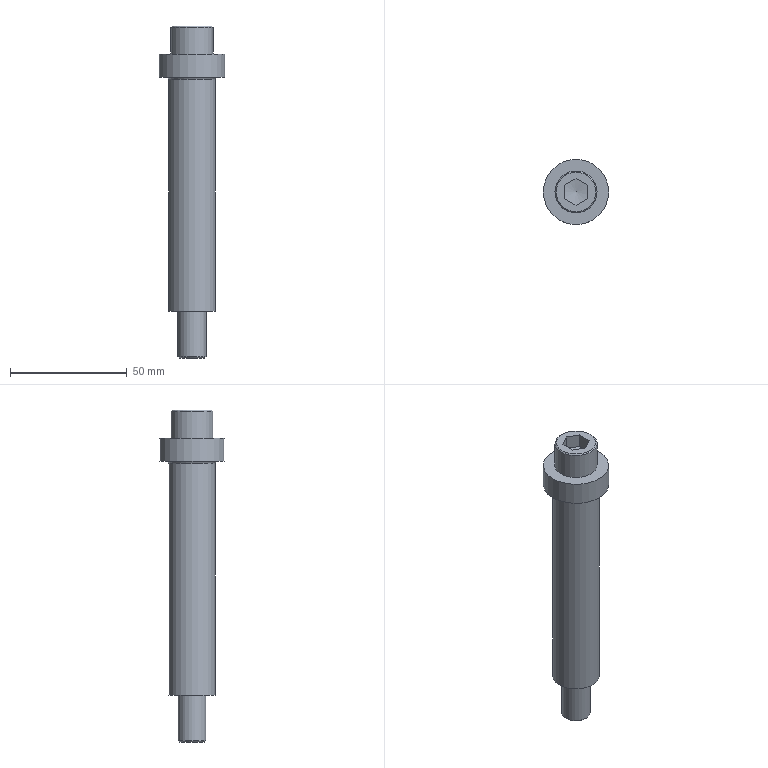Part | NX | features CSR20-100_1 2 | 1 solid | 27 faces | box 28 x 28 x 142 mm | volume 41062 mm3 | plane 18 | cylinder 5 | cone 3 | torus 1 | commonest cylinder face diameters 12 x1 12.6 x1 18 x1 20 x1 28 x1
STEP:
#1=CARTESIAN_POINT('',(1485.899,-26.667,139.999));
#2=VERTEX_POINT('',#1);
#3=CARTESIAN_POINT('',(1471.899,-26.667,139.999));
#4=DIRECTION('',(0.,0.,-1.));
#5=DIRECTION('',(1.,0.,0.));
#6=AXIS2_PLACEMENT_3D('',#3,#4,#5);
#7=CIRCLE('',#6,14.);
#8=EDGE_CURVE('',#2,#2,#7,.T.);
#9=ORIENTED_EDGE('',*,*,#8,.F.);
#10=EDGE_LOOP('',(#9));
#11=FACE_BOUND('',#10,.T.);
#12=CARTESIAN_POINT('',(1480.899,-26.667,139.999));
#13=VERTEX_POINT('',#12);
#14=CARTESIAN_POINT('',(1471.899,-26.667,139.999));
#15=DIRECTION('',(0.,0.,1.));
#16=DIRECTION('',(1.,0.,0.));
#17=AXIS2_PLACEMENT_3D('',#14,#15,#16);
#18=CIRCLE('',#17,9.);
#19=EDGE_CURVE('',#13,#13,#18,.T.);
#20=ORIENTED_EDGE('',*,*,#19,.F.);
#21=EDGE_LOOP('',(#20));
#22=FACE_BOUND('',#21,.T.);
#23=CARTESIAN_POINT('',(1471.899,-26.667,139.999));
#24=DIRECTION('',(0.,0.,1.));
#25=DIRECTION('',(1.,0.,0.));
#26=AXIS2_PLACEMENT_3D('',#23,#24,#25);
#27=PLANE('',#26);
#28=ADVANCED_FACE('',(#11,#22),#27,.T.);
#29=CARTESIAN_POINT('',(1481.899,-26.667,29.999));
#30=VERTEX_POINT('',#29);
#31=CARTESIAN_POINT('',(1471.899,-26.667,29.999));
#32=DIRECTION('',(0.,0.,1.));
#33=DIRECTION('',(1.,0.,0.));
#34=AXIS2_PLACEMENT_3D('',#31,#32,#33);
#35=CIRCLE('',#34,10.);
#36=EDGE_CURVE('',#30,#30,#35,.T.);
#37=ORIENTED_EDGE('',*,*,#36,.T.);
#38=EDGE_LOOP('',(#37));
#39=FACE_BOUND('',#38,.T.);
#40=CARTESIAN_POINT('',(1481.899,-26.667,128.999));
#41=VERTEX_POINT('',#40);
#42=CARTESIAN_POINT('',(1471.899,-26.667,128.999));
#43=DIRECTION('',(0.,0.,-1.));
#44=DIRECTION('',(-1.,0.,0.));
#45=AXIS2_PLACEMENT_3D('',#42,#43,#44);
#46=CIRCLE('',#45,10.);
#47=EDGE_CURVE('',#41,#41,#46,.T.);
#48=ORIENTED_EDGE('',*,*,#47,.T.);
#49=EDGE_LOOP('',(#48));
#50=FACE_BOUND('',#49,.T.);
#51=CARTESIAN_POINT('',(1471.899,-26.667,79.999));
#52=DIRECTION('',(0.,0.,-1.));
#53=DIRECTION('',(-1.,0.,0.));
#54=AXIS2_PLACEMENT_3D('',#51,#52,#53);
#55=CYLINDRICAL_SURFACE('',#54,10.);
#56=ADVANCED_FACE('',(#39,#50),#55,.T.);
#57=CARTESIAN_POINT('',(1478.199,-26.667,139.999));
#58=VERTEX_POINT('',#57);
#59=CARTESIAN_POINT('',(1471.899,-26.667,139.999));
#60=DIRECTION('',(0.,0.,1.));
#61=DIRECTION('',(1.,0.,0.));
#62=AXIS2_PLACEMENT_3D('',#59,#60,#61);
#63=CIRCLE('',#62,6.3);
#64=EDGE_CURVE('',#58,#58,#63,.T.);
#65=ORIENTED_EDGE('',*,*,#64,.T.);
#66=EDGE_LOOP('',(#65));
#67=FACE_BOUND('',#66,.T.);
#68=CARTESIAN_POINT('',(1478.199,-26.667,29.999));
#69=VERTEX_POINT('',#68);
#70=CARTESIAN_POINT('',(1471.899,-26.667,29.999));
#71=DIRECTION('',(0.,0.,-1.));
#72=DIRECTION('',(1.,0.,0.));
#73=AXIS2_PLACEMENT_3D('',#70,#71,#72);
#74=CIRCLE('',#73,6.3);
#75=EDGE_CURVE('',#69,#69,#74,.T.);
#76=ORIENTED_EDGE('',*,*,#75,.T.);
#77=EDGE_LOOP('',(#76));
#78=FACE_BOUND('',#77,.T.);
#79=CARTESIAN_POINT('',(1471.899,-26.667,84.999));
#80=DIRECTION('',(0.,0.,-1.));
#81=DIRECTION('',(-1.,0.,0.));
#82=AXIS2_PLACEMENT_3D('',#79,#80,#81);
#83=CYLINDRICAL_SURFACE('',#82,6.3);
#84=ADVANCED_FACE('',(#67,#78),#83,.F.);
#85=ORIENTED_EDGE('',*,*,#47,.F.);
#86=EDGE_LOOP('',(#85));
#87=FACE_BOUND('',#86,.T.);
#88=CARTESIAN_POINT('',(1482.899,-26.667,129.999));
#89=VERTEX_POINT('',#88);
#90=CARTESIAN_POINT('',(1471.899,-26.667,129.999));
#91=DIRECTION('',(0.,0.,1.));
#92=DIRECTION('',(-1.,0.,0.));
#93=AXIS2_PLACEMENT_3D('',#90,#91,#92);
#94=CIRCLE('',#93,11.);
#95=EDGE_CURVE('',#89,#89,#94,.T.);
#96=ORIENTED_EDGE('',*,*,#95,.F.);
#97=EDGE_LOOP('',(#96));
#98=FACE_BOUND('',#97,.T.);
#99=CARTESIAN_POINT('',(1471.899,-26.667,128.999));
#100=DIRECTION('',(0.,0.,1.));
#101=DIRECTION('',(1.,0.,0.));
#102=AXIS2_PLACEMENT_3D('',#99,#100,#101);
#103=TOROIDAL_SURFACE('',#102,11.,1.);
#104=ADVANCED_FACE('',(#87,#98),#103,.F.);
#105=CARTESIAN_POINT('',(1485.899,-26.667,129.999));
#106=VERTEX_POINT('',#105);
#107=CARTESIAN_POINT('',(1471.899,-26.667,129.999));
#108=DIRECTION('',(0.,0.,1.));
#109=DIRECTION('',(1.,0.,0.));
#110=AXIS2_PLACEMENT_3D('',#107,#108,#109);
#111=CIRCLE('',#110,14.);
#112=EDGE_CURVE('',#106,#106,#111,.T.);
#113=ORIENTED_EDGE('',*,*,#112,.F.);
#114=EDGE_LOOP('',(#113));
#115=FACE_BOUND('',#114,.T.);
#116=ORIENTED_EDGE('',*,*,#95,.T.);
#117=EDGE_LOOP('',(#116));
#118=FACE_BOUND('',#117,.T.);
#119=CARTESIAN_POINT('',(1471.899,-26.667,129.999));
#120=DIRECTION('',(0.,0.,-1.));
#121=DIRECTION('',(-1.,0.,0.));
#122=AXIS2_PLACEMENT_3D('',#119,#120,#121);
#123=PLANE('',#122);
#124=ADVANCED_FACE('',(#115,#118),#123,.T.);
#125=ORIENTED_EDGE('',*,*,#75,.F.);
#126=EDGE_LOOP('',(#125));
#127=FACE_BOUND('',#126,.T.);
#128=ORIENTED_EDGE('',*,*,#36,.F.);
#129=EDGE_LOOP('',(#128));
#130=FACE_BOUND('',#129,.T.);
#131=CARTESIAN_POINT('',(1471.899,-26.667,29.999));
#132=DIRECTION('',(0.,0.,-1.));
#133=DIRECTION('',(-1.,0.,0.));
#134=AXIS2_PLACEMENT_3D('',#131,#132,#133);
#135=PLANE('',#134);
#136=ADVANCED_FACE('',(#127,#130),#135,.T.);
#137=ORIENTED_EDGE('',*,*,#8,.T.);
#138=EDGE_LOOP('',(#137));
#139=FACE_BOUND('',#138,.T.);
#140=ORIENTED_EDGE('',*,*,#112,.T.);
#141=EDGE_LOOP('',(#140));
#142=FACE_BOUND('',#141,.T.);
#143=CARTESIAN_POINT('',(1471.899,-26.667,134.999));
#144=DIRECTION('',(0.,0.,-1.));
#145=DIRECTION('',(-1.,0.,0.));
#146=AXIS2_PLACEMENT_3D('',#143,#144,#145);
#147=CYLINDRICAL_SURFACE('',#146,14.);
#148=ADVANCED_FACE('',(#139,#142),#147,.T.);
#149=CARTESIAN_POINT('',(1471.899,-32.441,151.999));
#150=VERTEX_POINT('',#149);
#151=CARTESIAN_POINT('',(1476.899,-29.554,151.999));
#152=VERTEX_POINT('',#151);
#153=CARTESIAN_POINT('',(1474.399,-30.997,151.999));
#154=DIRECTION('',(0.866,0.5,0.));
#155=VECTOR('',#154,1000.);
#156=LINE('',#153,#155);
#157=EDGE_CURVE('',#150,#152,#156,.T.);
#158=ORIENTED_EDGE('',*,*,#157,.F.);
#159=CARTESIAN_POINT('',(1466.899,-29.554,151.999));
#160=VERTEX_POINT('',#159);
#161=CARTESIAN_POINT('',(1469.399,-30.997,151.999));
#162=DIRECTION('',(0.866,-0.5,0.));
#163=VECTOR('',#162,1000.);
#164=LINE('',#161,#163);
#165=EDGE_CURVE('',#160,#150,#164,.T.);
#166=ORIENTED_EDGE('',*,*,#165,.F.);
#167=CARTESIAN_POINT('',(1466.899,-23.78,151.999));
#168=VERTEX_POINT('',#167);
#169=CARTESIAN_POINT('',(1466.899,-26.667,151.999));
#170=DIRECTION('',(0.,-1.,0.));
#171=VECTOR('',#170,1000.);
#172=LINE('',#169,#171);
#173=EDGE_CURVE('',#168,#160,#172,.T.);
#174=ORIENTED_EDGE('',*,*,#173,.F.);
#175=CARTESIAN_POINT('',(1471.899,-20.894,151.999));
#176=VERTEX_POINT('',#175);
#177=CARTESIAN_POINT('',(1469.399,-22.337,151.999));
#178=DIRECTION('',(-0.866,-0.5,0.));
#179=VECTOR('',#178,1000.);
#180=LINE('',#177,#179);
#181=EDGE_CURVE('',#176,#168,#180,.T.);
#182=ORIENTED_EDGE('',*,*,#181,.F.);
#183=CARTESIAN_POINT('',(1476.899,-23.78,151.999));
#184=VERTEX_POINT('',#183);
#185=CARTESIAN_POINT('',(1474.399,-22.337,151.999));
#186=DIRECTION('',(-0.866,0.5,0.));
#187=VECTOR('',#186,1000.);
#188=LINE('',#185,#187);
#189=EDGE_CURVE('',#184,#176,#188,.T.);
#190=ORIENTED_EDGE('',*,*,#189,.F.);
#191=CARTESIAN_POINT('',(1476.899,-26.667,151.999));
#192=DIRECTION('',(0.,1.,0.));
#193=VECTOR('',#192,1000.);
#194=LINE('',#191,#193);
#195=EDGE_CURVE('',#152,#184,#194,.T.);
#196=ORIENTED_EDGE('',*,*,#195,.F.);
#197=EDGE_LOOP('',(#158,#166,#174,#182,#190,#196));
#198=FACE_BOUND('',#197,.T.);
#199=CARTESIAN_POINT('',(1480.399,-26.667,151.999));
#200=VERTEX_POINT('',#199);
#201=CARTESIAN_POINT('',(1471.899,-26.667,151.999));
#202=DIRECTION('',(0.,0.,1.));
#203=DIRECTION('',(-1.,0.,0.));
#204=AXIS2_PLACEMENT_3D('',#201,#202,#203);
#205=CIRCLE('',#204,8.5);
#206=EDGE_CURVE('',#200,#200,#205,.T.);
#207=ORIENTED_EDGE('',*,*,#206,.T.);
#208=EDGE_LOOP('',(#207));
#209=FACE_BOUND('',#208,.T.);
#210=CARTESIAN_POINT('',(1471.899,-26.667,151.999));
#211=DIRECTION('',(0.,0.,1.));
#212=DIRECTION('',(1.,0.,0.));
#213=AXIS2_PLACEMENT_3D('',#210,#211,#212);
#214=PLANE('',#213);
#215=ADVANCED_FACE('',(#198,#209),#214,.T.);
#216=ORIENTED_EDGE('',*,*,#19,.T.);
#217=EDGE_LOOP('',(#216));
#218=FACE_BOUND('',#217,.T.);
#219=CARTESIAN_POINT('',(1480.899,-26.667,151.499));
#220=VERTEX_POINT('',#219);
#221=CARTESIAN_POINT('',(1471.899,-26.667,151.499));
#222=DIRECTION('',(0.,0.,-1.));
#223=DIRECTION('',(-1.,0.,0.));
#224=AXIS2_PLACEMENT_3D('',#221,#222,#223);
#225=CIRCLE('',#224,9.);
#226=EDGE_CURVE('',#220,#220,#225,.T.);
#227=ORIENTED_EDGE('',*,*,#226,.T.);
#228=EDGE_LOOP('',(#227));
#229=FACE_BOUND('',#228,.T.);
#230=CARTESIAN_POINT('',(1471.899,-26.667,145.999));
#231=DIRECTION('',(0.,0.,-1.));
#232=DIRECTION('',(-1.,0.,0.));
#233=AXIS2_PLACEMENT_3D('',#230,#231,#232);
#234=CYLINDRICAL_SURFACE('',#233,9.);
#235=ADVANCED_FACE('',(#218,#229),#234,.T.);
#236=ORIENTED_EDGE('',*,*,#226,.F.);
#237=EDGE_LOOP('',(#236));
#238=FACE_BOUND('',#237,.T.);
#239=ORIENTED_EDGE('',*,*,#206,.F.);
#240=EDGE_LOOP('',(#239));
#241=FACE_BOUND('',#240,.T.);
#242=CARTESIAN_POINT('',(1471.899,-26.667,151.999));
#243=DIRECTION('',(0.,0.,-1.));
#244=DIRECTION('',(1.,0.,0.));
#245=AXIS2_PLACEMENT_3D('',#242,#243,#244);
#246=CONICAL_SURFACE('',#245,8.5,0.7854);
#247=ADVANCED_FACE('',(#238,#241),#246,.T.);
#248=CARTESIAN_POINT('',(1476.899,-29.554,145.999));
#249=VERTEX_POINT('',#248);
#250=CARTESIAN_POINT('',(1476.899,-29.554,148.999));
#251=DIRECTION('',(0.,0.,1.));
#252=VECTOR('',#251,1000.);
#253=LINE('',#250,#252);
#254=EDGE_CURVE('',#249,#152,#253,.T.);
#255=ORIENTED_EDGE('',*,*,#254,.T.);
#256=ORIENTED_EDGE('',*,*,#195,.T.);
#257=CARTESIAN_POINT('',(1476.899,-23.78,145.999));
#258=VERTEX_POINT('',#257);
#259=CARTESIAN_POINT('',(1476.899,-23.78,148.999));
#260=DIRECTION('',(0.,0.,1.));
#261=VECTOR('',#260,1000.);
#262=LINE('',#259,#261);
#263=EDGE_CURVE('',#258,#184,#262,.T.);
#264=ORIENTED_EDGE('',*,*,#263,.F.);
#265=CARTESIAN_POINT('',(1476.899,-26.667,145.999));
#266=DIRECTION('',(0.,1.,0.));
#267=VECTOR('',#266,1000.);
#268=LINE('',#265,#267);
#269=EDGE_CURVE('',#249,#258,#268,.T.);
#270=ORIENTED_EDGE('',*,*,#269,.F.);
#271=EDGE_LOOP('',(#255,#256,#264,#270));
#272=FACE_BOUND('',#271,.T.);
#273=CARTESIAN_POINT('',(1476.899,-26.667,148.999));
#274=DIRECTION('',(-1.,0.,0.));
#275=DIRECTION('',(0.,0.,1.));
#276=AXIS2_PLACEMENT_3D('',#273,#274,#275);
#277=PLANE('',#276);
#278=ADVANCED_FACE('',(#272),#277,.T.);
#279=ORIENTED_EDGE('',*,*,#263,.T.);
#280=ORIENTED_EDGE('',*,*,#189,.T.);
#281=CARTESIAN_POINT('',(1471.899,-20.894,145.999));
#282=VERTEX_POINT('',#281);
#283=CARTESIAN_POINT('',(1471.899,-20.894,148.999));
#284=DIRECTION('',(0.,0.,1.));
#285=VECTOR('',#284,1000.);
#286=LINE('',#283,#285);
#287=EDGE_CURVE('',#282,#176,#286,.T.);
#288=ORIENTED_EDGE('',*,*,#287,.F.);
#289=CARTESIAN_POINT('',(1474.399,-22.337,145.999));
#290=DIRECTION('',(-0.866,0.5,0.));
#291=VECTOR('',#290,1000.);
#292=LINE('',#289,#291);
#293=EDGE_CURVE('',#258,#282,#292,.T.);
#294=ORIENTED_EDGE('',*,*,#293,.F.);
#295=EDGE_LOOP('',(#279,#280,#288,#294));
#296=FACE_BOUND('',#295,.T.);
#297=CARTESIAN_POINT('',(1474.399,-22.337,148.999));
#298=DIRECTION('',(-0.5,-0.866,0.));
#299=DIRECTION('',(0.,0.,1.));
#300=AXIS2_PLACEMENT_3D('',#297,#298,#299);
#301=PLANE('',#300);
#302=ADVANCED_FACE('',(#296),#301,.T.);
#303=ORIENTED_EDGE('',*,*,#287,.T.);
#304=ORIENTED_EDGE('',*,*,#181,.T.);
#305=CARTESIAN_POINT('',(1466.899,-23.78,145.999));
#306=VERTEX_POINT('',#305);
#307=CARTESIAN_POINT('',(1466.899,-23.78,148.999));
#308=DIRECTION('',(0.,0.,1.));
#309=VECTOR('',#308,1000.);
#310=LINE('',#307,#309);
#311=EDGE_CURVE('',#306,#168,#310,.T.);
#312=ORIENTED_EDGE('',*,*,#311,.F.);
#313=CARTESIAN_POINT('',(1469.399,-22.337,145.999));
#314=DIRECTION('',(-0.866,-0.5,0.));
#315=VECTOR('',#314,1000.);
#316=LINE('',#313,#315);
#317=EDGE_CURVE('',#282,#306,#316,.T.);
#318=ORIENTED_EDGE('',*,*,#317,.F.);
#319=EDGE_LOOP('',(#303,#304,#312,#318));
#320=FACE_BOUND('',#319,.T.);
#321=CARTESIAN_POINT('',(1469.399,-22.337,148.999));
#322=DIRECTION('',(0.5,-0.866,0.));
#323=DIRECTION('',(0.,0.,-1.));
#324=AXIS2_PLACEMENT_3D('',#321,#322,#323);
#325=PLANE('',#324);
#326=ADVANCED_FACE('',(#320),#325,.T.);
#327=ORIENTED_EDGE('',*,*,#311,.T.);
#328=ORIENTED_EDGE('',*,*,#173,.T.);
#329=CARTESIAN_POINT('',(1466.899,-29.554,145.999));
#330=VERTEX_POINT('',#329);
#331=CARTESIAN_POINT('',(1466.899,-29.554,148.999));
#332=DIRECTION('',(0.,0.,1.));
#333=VECTOR('',#332,1000.);
#334=LINE('',#331,#333);
#335=EDGE_CURVE('',#330,#160,#334,.T.);
#336=ORIENTED_EDGE('',*,*,#335,.F.);
#337=CARTESIAN_POINT('',(1466.899,-26.667,145.999));
#338=DIRECTION('',(0.,-1.,0.));
#339=VECTOR('',#338,1000.);
#340=LINE('',#337,#339);
#341=EDGE_CURVE('',#306,#330,#340,.T.);
#342=ORIENTED_EDGE('',*,*,#341,.F.);
#343=EDGE_LOOP('',(#327,#328,#336,#342));
#344=FACE_BOUND('',#343,.T.);
#345=CARTESIAN_POINT('',(1466.899,-26.667,148.999));
#346=DIRECTION('',(1.,0.,0.));
#347=DIRECTION('',(0.,0.,-1.));
#348=AXIS2_PLACEMENT_3D('',#345,#346,#347);
#349=PLANE('',#348);
#350=ADVANCED_FACE('',(#344),#349,.T.);
#351=ORIENTED_EDGE('',*,*,#335,.T.);
#352=ORIENTED_EDGE('',*,*,#165,.T.);
#353=CARTESIAN_POINT('',(1471.899,-32.441,145.999));
#354=VERTEX_POINT('',#353);
#355=CARTESIAN_POINT('',(1471.899,-32.441,148.999));
#356=DIRECTION('',(0.,0.,1.));
#357=VECTOR('',#356,1000.);
#358=LINE('',#355,#357);
#359=EDGE_CURVE('',#354,#150,#358,.T.);
#360=ORIENTED_EDGE('',*,*,#359,.F.);
#361=CARTESIAN_POINT('',(1469.399,-30.997,145.999));
#362=DIRECTION('',(0.866,-0.5,0.));
#363=VECTOR('',#362,1000.);
#364=LINE('',#361,#363);
#365=EDGE_CURVE('',#330,#354,#364,.T.);
#366=ORIENTED_EDGE('',*,*,#365,.F.);
#367=EDGE_LOOP('',(#351,#352,#360,#366));
#368=FACE_BOUND('',#367,.T.);
#369=CARTESIAN_POINT('',(1469.399,-30.997,148.999));
#370=DIRECTION('',(0.5,0.866,0.));
#371=DIRECTION('',(0.,0.,-1.));
#372=AXIS2_PLACEMENT_3D('',#369,#370,#371);
#373=PLANE('',#372);
#374=ADVANCED_FACE('',(#368),#373,.T.);
#375=ORIENTED_EDGE('',*,*,#359,.T.);
#376=ORIENTED_EDGE('',*,*,#157,.T.);
#377=ORIENTED_EDGE('',*,*,#254,.F.);
#378=CARTESIAN_POINT('',(1474.399,-30.997,145.999));
#379=DIRECTION('',(0.866,0.5,0.));
#380=VECTOR('',#379,1000.);
#381=LINE('',#378,#380);
#382=EDGE_CURVE('',#354,#249,#381,.T.);
#383=ORIENTED_EDGE('',*,*,#382,.F.);
#384=EDGE_LOOP('',(#375,#376,#377,#383));
#385=FACE_BOUND('',#384,.T.);
#386=CARTESIAN_POINT('',(1474.399,-30.997,148.999));
#387=DIRECTION('',(-0.5,0.866,0.));
#388=DIRECTION('',(0.,0.,1.));
#389=AXIS2_PLACEMENT_3D('',#386,#387,#388);
#390=PLANE('',#389);
#391=ADVANCED_FACE('',(#385),#390,.T.);
#392=CARTESIAN_POINT('',(1471.899,-26.667,145.999));
#393=DIRECTION('',(0.,0.,-1.));
#394=DIRECTION('',(1.,0.,0.));
#395=AXIS2_PLACEMENT_3D('',#392,#393,#394);
#396=CIRCLE('',#395,5.774);
#397=EDGE_CURVE('',#258,#249,#396,.T.);
#398=ORIENTED_EDGE('',*,*,#397,.F.);
#399=CARTESIAN_POINT('',(1471.899,-26.667,145.999));
#400=DIRECTION('',(0.,0.,-1.));
#401=DIRECTION('',(1.,0.,0.));
#402=AXIS2_PLACEMENT_3D('',#399,#400,#401);
#403=CIRCLE('',#402,5.774);
#404=EDGE_CURVE('',#282,#258,#403,.T.);
#405=ORIENTED_EDGE('',*,*,#404,.F.);
#406=CARTESIAN_POINT('',(1471.899,-26.667,145.999));
#407=DIRECTION('',(0.,0.,-1.));
#408=DIRECTION('',(1.,0.,0.));
#409=AXIS2_PLACEMENT_3D('',#406,#407,#408);
#410=CIRCLE('',#409,5.774);
#411=EDGE_CURVE('',#306,#282,#410,.T.);
#412=ORIENTED_EDGE('',*,*,#411,.F.);
#413=CARTESIAN_POINT('',(1471.899,-26.667,145.999));
#414=DIRECTION('',(0.,0.,-1.));
#415=DIRECTION('',(1.,0.,0.));
#416=AXIS2_PLACEMENT_3D('',#413,#414,#415);
#417=CIRCLE('',#416,5.774);
#418=EDGE_CURVE('',#330,#306,#417,.T.);
#419=ORIENTED_EDGE('',*,*,#418,.F.);
#420=CARTESIAN_POINT('',(1471.899,-26.667,145.999));
#421=DIRECTION('',(0.,0.,-1.));
#422=DIRECTION('',(1.,0.,0.));
#423=AXIS2_PLACEMENT_3D('',#420,#421,#422);
#424=CIRCLE('',#423,5.774);
#425=EDGE_CURVE('',#354,#330,#424,.T.);
#426=ORIENTED_EDGE('',*,*,#425,.F.);
#427=CARTESIAN_POINT('',(1471.899,-26.667,145.999));
#428=DIRECTION('',(0.,0.,-1.));
#429=DIRECTION('',(1.,0.,0.));
#430=AXIS2_PLACEMENT_3D('',#427,#428,#429);
#431=CIRCLE('',#430,5.774);
#432=EDGE_CURVE('',#249,#354,#431,.T.);
#433=ORIENTED_EDGE('',*,*,#432,.F.);
#434=EDGE_LOOP('',(#398,#405,#412,#419,#426,#433));
#435=FACE_BOUND('',#434,.T.);
#436=CARTESIAN_POINT('',(1471.899,-26.667,144.999));
#437=VERTEX_POINT('',#436);
#438=VERTEX_LOOP('',#437);
#439=FACE_BOUND('',#438,.T.);
#440=CARTESIAN_POINT('',(1471.899,-26.667,145.499));
#441=DIRECTION('',(0.,0.,1.));
#442=DIRECTION('',(-1.,0.,0.));
#443=AXIS2_PLACEMENT_3D('',#440,#441,#442);
#444=CONICAL_SURFACE('',#443,2.887,1.399);
#445=ADVANCED_FACE('',(#435,#439),#444,.F.);
#446=ORIENTED_EDGE('',*,*,#365,.T.);
#447=ORIENTED_EDGE('',*,*,#425,.T.);
#448=EDGE_LOOP('',(#446,#447));
#449=FACE_BOUND('',#448,.T.);
#450=CARTESIAN_POINT('',(1471.899,-26.667,145.999));
#451=DIRECTION('',(0.,0.,1.));
#452=DIRECTION('',(1.,0.,0.));
#453=AXIS2_PLACEMENT_3D('',#450,#451,#452);
#454=PLANE('',#453);
#455=ADVANCED_FACE('',(#449),#454,.F.);
#456=ORIENTED_EDGE('',*,*,#341,.T.);
#457=ORIENTED_EDGE('',*,*,#418,.T.);
#458=EDGE_LOOP('',(#456,#457));
#459=FACE_BOUND('',#458,.T.);
#460=CARTESIAN_POINT('',(1471.899,-26.667,145.999));
#461=DIRECTION('',(0.,0.,1.));
#462=DIRECTION('',(1.,0.,0.));
#463=AXIS2_PLACEMENT_3D('',#460,#461,#462);
#464=PLANE('',#463);
#465=ADVANCED_FACE('',(#459),#464,.F.);
#466=ORIENTED_EDGE('',*,*,#317,.T.);
#467=ORIENTED_EDGE('',*,*,#411,.T.);
#468=EDGE_LOOP('',(#466,#467));
#469=FACE_BOUND('',#468,.T.);
#470=CARTESIAN_POINT('',(1471.899,-26.667,145.999));
#471=DIRECTION('',(0.,0.,1.));
#472=DIRECTION('',(1.,0.,0.));
#473=AXIS2_PLACEMENT_3D('',#470,#471,#472);
#474=PLANE('',#473);
#475=ADVANCED_FACE('',(#469),#474,.F.);
#476=ORIENTED_EDGE('',*,*,#293,.T.);
#477=ORIENTED_EDGE('',*,*,#404,.T.);
#478=EDGE_LOOP('',(#476,#477));
#479=FACE_BOUND('',#478,.T.);
#480=CARTESIAN_POINT('',(1471.899,-26.667,145.999));
#481=DIRECTION('',(0.,0.,1.));
#482=DIRECTION('',(1.,0.,0.));
#483=AXIS2_PLACEMENT_3D('',#480,#481,#482);
#484=PLANE('',#483);
#485=ADVANCED_FACE('',(#479),#484,.F.);
#486=ORIENTED_EDGE('',*,*,#269,.T.);
#487=ORIENTED_EDGE('',*,*,#397,.T.);
#488=EDGE_LOOP('',(#486,#487));
#489=FACE_BOUND('',#488,.T.);
#490=CARTESIAN_POINT('',(1471.899,-26.667,145.999));
#491=DIRECTION('',(0.,0.,1.));
#492=DIRECTION('',(1.,0.,0.));
#493=AXIS2_PLACEMENT_3D('',#490,#491,#492);
#494=PLANE('',#493);
#495=ADVANCED_FACE('',(#489),#494,.F.);
#496=ORIENTED_EDGE('',*,*,#382,.T.);
#497=ORIENTED_EDGE('',*,*,#432,.T.);
#498=EDGE_LOOP('',(#496,#497));
#499=FACE_BOUND('',#498,.T.);
#500=CARTESIAN_POINT('',(1471.899,-26.667,145.999));
#501=DIRECTION('',(0.,0.,1.));
#502=DIRECTION('',(1.,0.,0.));
#503=AXIS2_PLACEMENT_3D('',#500,#501,#502);
#504=PLANE('',#503);
#505=ADVANCED_FACE('',(#499),#504,.F.);
#506=CARTESIAN_POINT('',(1477.899,-26.667,10.499));
#507=VERTEX_POINT('',#506);
#508=CARTESIAN_POINT('',(1471.899,-26.667,10.499));
#509=DIRECTION('',(0.,0.,1.));
#510=DIRECTION('',(-1.,0.,0.));
#511=AXIS2_PLACEMENT_3D('',#508,#509,#510);
#512=CIRCLE('',#511,6.);
#513=EDGE_CURVE('',#507,#507,#512,.T.);
#514=ORIENTED_EDGE('',*,*,#513,.F.);
#515=EDGE_LOOP('',(#514));
#516=FACE_BOUND('',#515,.T.);
#517=CARTESIAN_POINT('',(1477.399,-26.667,9.999));
#518=VERTEX_POINT('',#517);
#519=CARTESIAN_POINT('',(1471.899,-26.667,9.999));
#520=DIRECTION('',(0.,0.,-1.));
#521=DIRECTION('',(-1.,0.,0.));
#522=AXIS2_PLACEMENT_3D('',#519,#520,#521);
#523=CIRCLE('',#522,5.5);
#524=EDGE_CURVE('',#518,#518,#523,.T.);
#525=ORIENTED_EDGE('',*,*,#524,.F.);
#526=EDGE_LOOP('',(#525));
#527=FACE_BOUND('',#526,.T.);
#528=CARTESIAN_POINT('',(1471.899,-26.667,9.999));
#529=DIRECTION('',(0.,0.,1.));
#530=DIRECTION('',(1.,0.,0.));
#531=AXIS2_PLACEMENT_3D('',#528,#529,#530);
#532=CONICAL_SURFACE('',#531,5.5,0.7854);
#533=ADVANCED_FACE('',(#516,#527),#532,.T.);
#534=CARTESIAN_POINT('',(1477.899,-26.667,139.999));
#535=VERTEX_POINT('',#534);
#536=CARTESIAN_POINT('',(1471.899,-26.667,139.999));
#537=DIRECTION('',(0.,0.,-1.));
#538=DIRECTION('',(1.,0.,0.));
#539=AXIS2_PLACEMENT_3D('',#536,#537,#538);
#540=CIRCLE('',#539,6.);
#541=EDGE_CURVE('',#535,#535,#540,.T.);
#542=ORIENTED_EDGE('',*,*,#541,.T.);
#543=EDGE_LOOP('',(#542));
#544=FACE_BOUND('',#543,.T.);
#545=ORIENTED_EDGE('',*,*,#513,.T.);
#546=EDGE_LOOP('',(#545));
#547=FACE_BOUND('',#546,.T.);
#548=CARTESIAN_POINT('',(1471.899,-26.667,74.999));
#549=DIRECTION('',(0.,0.,-1.));
#550=DIRECTION('',(-1.,0.,0.));
#551=AXIS2_PLACEMENT_3D('',#548,#549,#550);
#552=CYLINDRICAL_SURFACE('',#551,6.);
#553=ADVANCED_FACE('',(#544,#547),#552,.T.);
#554=ORIENTED_EDGE('',*,*,#524,.T.);
#555=EDGE_LOOP('',(#554));
#556=FACE_BOUND('',#555,.T.);
#557=CARTESIAN_POINT('',(1471.899,-26.667,9.999));
#558=DIRECTION('',(0.,0.,-1.));
#559=DIRECTION('',(-1.,0.,0.));
#560=AXIS2_PLACEMENT_3D('',#557,#558,#559);
#561=PLANE('',#560);
#562=ADVANCED_FACE('',(#556),#561,.T.);
#563=ORIENTED_EDGE('',*,*,#64,.F.);
#564=EDGE_LOOP('',(#563));
#565=FACE_BOUND('',#564,.T.);
#566=ORIENTED_EDGE('',*,*,#541,.F.);
#567=EDGE_LOOP('',(#566));
#568=FACE_BOUND('',#567,.T.);
#569=CARTESIAN_POINT('',(1471.899,-26.667,139.999));
#570=DIRECTION('',(0.,0.,-1.));
#571=DIRECTION('',(-1.,0.,0.));
#572=AXIS2_PLACEMENT_3D('',#569,#570,#571);
#573=PLANE('',#572);
#574=ADVANCED_FACE('',(#565,#568),#573,.T.);
#575=CLOSED_SHELL('',(#28,#56,#84,#104,#124,#136,#148,#215,#235,#247,#278,#302,#326,#350,#374,#391,#445,#455,#465,#475,#485,#495,#505,#533,#553,#562,#574));
#576=MANIFOLD_SOLID_BREP('',#575);
#577=(LENGTH_UNIT()NAMED_UNIT(*)SI_UNIT(.MILLI.,.METRE.));
#578=UNCERTAINTY_MEASURE_WITH_UNIT(LENGTH_MEASURE(0.00001),#577,'','');
#579=(NAMED_UNIT(*)PLANE_ANGLE_UNIT()SI_UNIT($,.RADIAN.));
#580=(NAMED_UNIT(*)SI_UNIT($,.STERADIAN.)SOLID_ANGLE_UNIT());
#581=(GEOMETRIC_REPRESENTATION_CONTEXT(3)GLOBAL_UNCERTAINTY_ASSIGNED_CONTEXT((#578))GLOBAL_UNIT_ASSIGNED_CONTEXT((#577,#579,#580))REPRESENTATION_CONTEXT('',''));
#582=ADVANCED_BREP_SHAPE_REPRESENTATION('',(#576),#581);